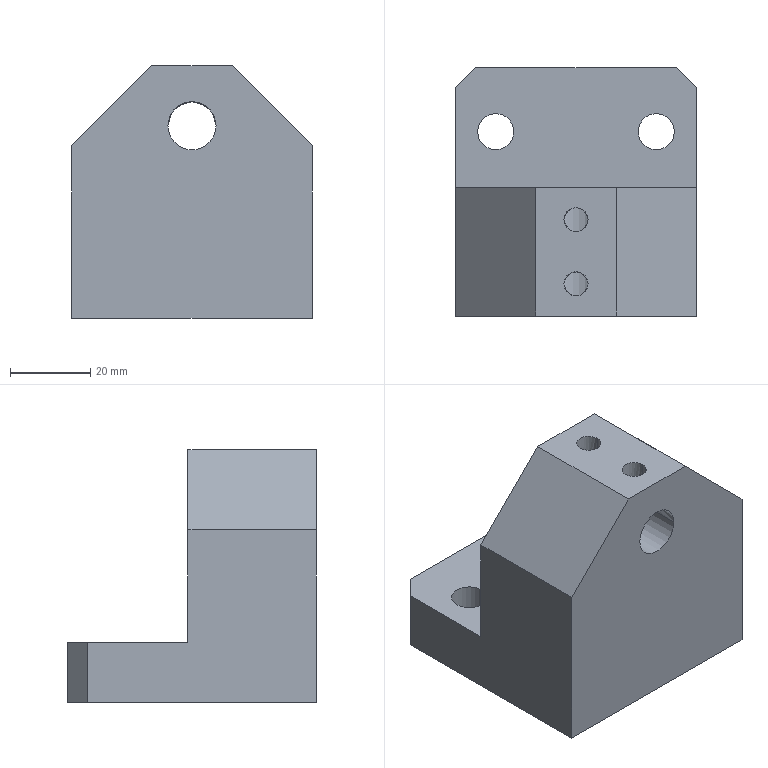Part | STEP file | GUIDE.HOLDER.stp | 1 solid | 22 faces | box 60 x 62 x 63 mm | volume 128733 mm3 | spline 18 | plane 4